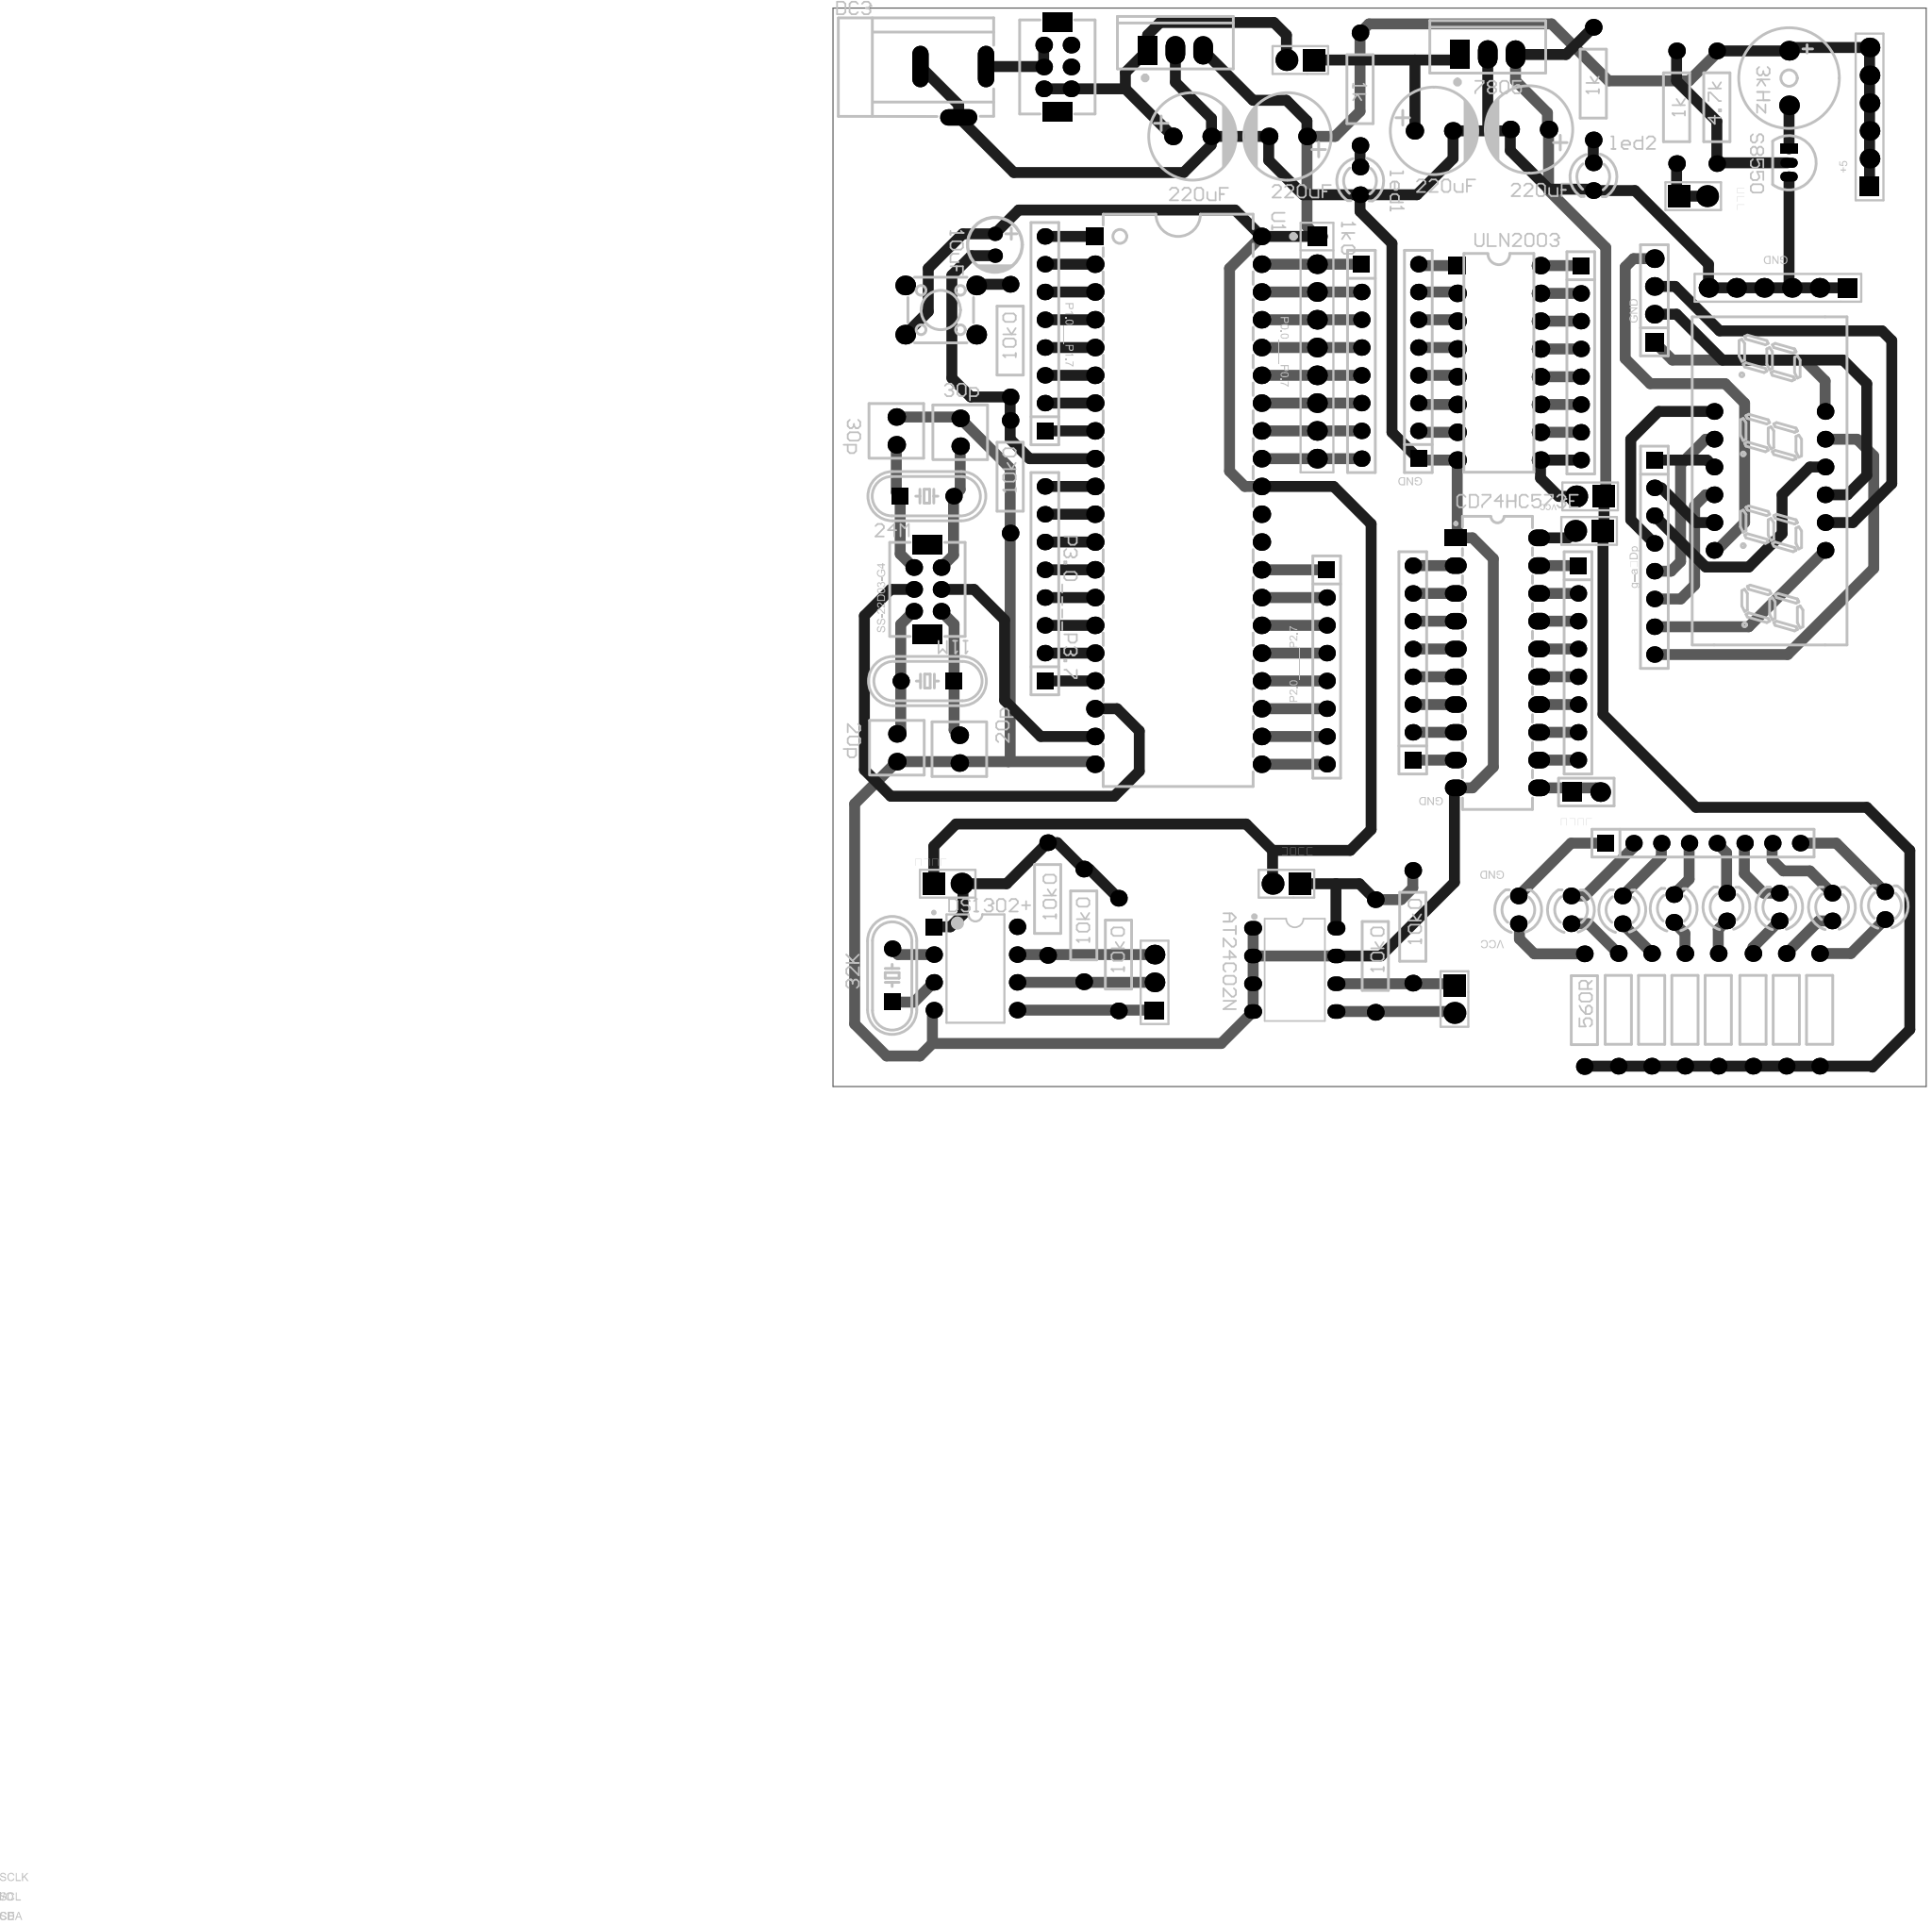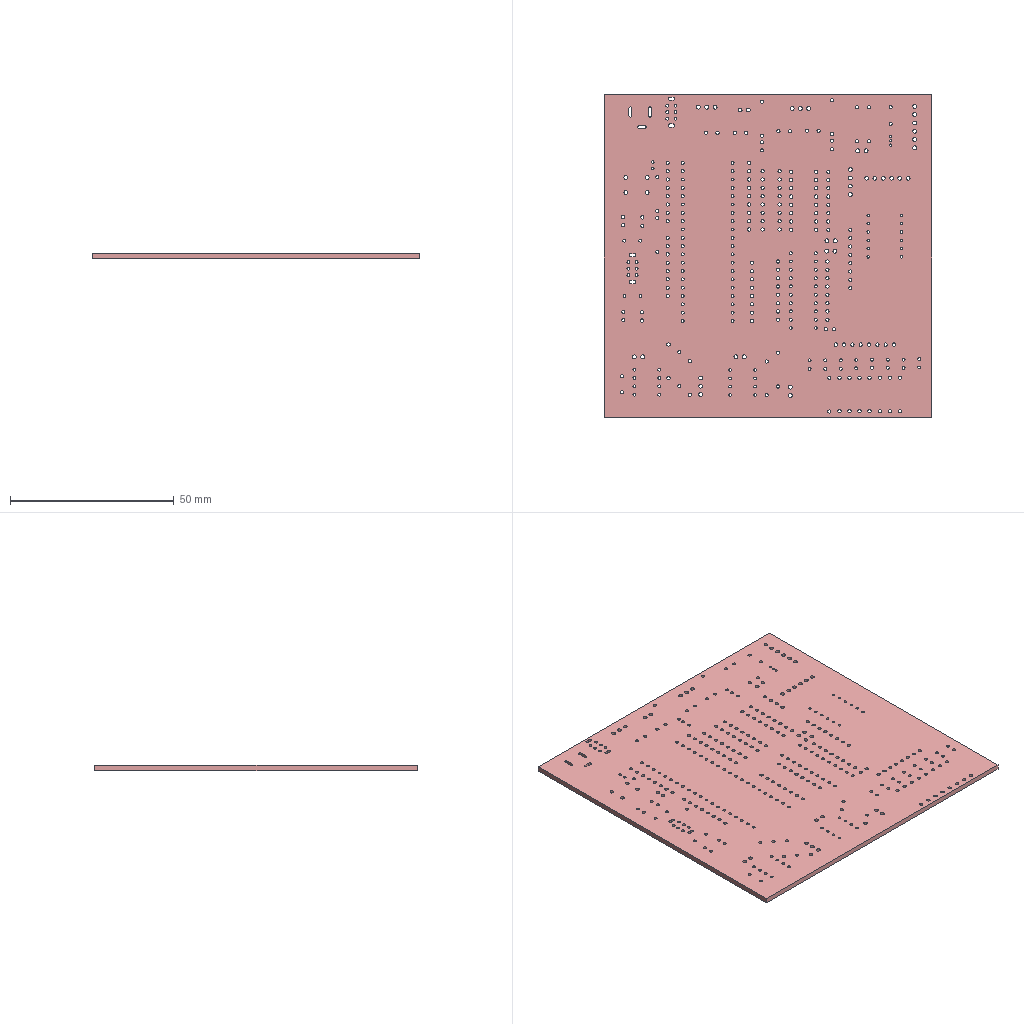Circuit board layout | Altium Designer | box 100 x 98.6 x 1.6 mm
Layer stack:
# Altium Designer layer stack of  (unit mm; dielectric type: 0 none, 1 core, 2 prepreg, 3 surface material)
index,name,kind,layer,copper_thickness_mm,dielectric_type,dielectric_thickness_mm,dielectric_material,dielectric_constant
0,Top Paste Mask Layer,other,,,,,,
1,Top Silkscreen Layer,other,,,,,,
2,Top Solder Mask Layer,dielectric,,,3,0.01,,3.3
3,Top Layer,copper,Top Layer,0.035,,,,
4,Dielectric1,dielectric,,,3,1.51,FR4,4.5
5,Bottom Layer,copper,Bottom Layer,0.035,,,,
6,Bottom Solder Mask Layer,dielectric,,,3,0.01,,3.3
7,Bottom Silkscreen Layer,other,,,,,,
8,Bottom Paste Mask Layer,other,,,,,,
# drill layer pairs: low layer,high layer
drill_pair,Top Layer,Bottom Layer
Part placement:
Designator,Comment,Layer,Footprint,Center-X(mm),Center-Y(mm),Rotation
H31,PZ254V-11-02P,TopLayer,HDR-TH_2P-P2.54-V-M,145.364,127,180
U1,STC89C52RC-40I-PDIP40,TopLayer,DIP-40_L52.0-W13.7-P2.54-LS15.2-BL,107.772,129.794,270
H32,PZ254V-11-02P,TopLayer,HDR-TH_2P-P2.54-V-M,145.458,130.153,180
Q1,ULN2003,TopLayer,DIP-16_L19.8-W6.5-P2.54-LS7.6-BL,137.109,142.367,270
U2,7805,TopLayer,TO-220-3_L10.0-W4.5-P2.54-L,136.093,170.561,0
U3,7805,TopLayer,TO-220-3_L10.0-W4.5-P2.54-L,107.518,170.942,0
U4,DS1302+,TopLayer,DIP-8_L9.8-W6.6-P2.54-LS7.6-BL,89.23,86.995,270
X1,24M,TopLayer,HC-49US_L11.5-W4.5-P4.88,84.785,130.175,0
U5,AT24C02N,TopLayer,DIP-8_L9.2-W6.3-P2.54-LS7.62-BL,118.44,86.868,270
U6,CD74HC573E,TopLayer,DIP-20_L26.8-W6.4-P2.54-LS7.6-BL,136.982,114.935,270
BUZZER1,3kHz,TopLayer,BUZ-TH_BD9.0-P5.00-D0.6-FD,163.652,168.402,270
H16,P3.0____P3.7,TopLayer,HDR-TH_8P-P2.54-V-M,95.58,122.174,90
Q2,S8550,TopLayer,TO-92-3_L4.9-W3.7-P1.27-L,163.652,160.655,270
C1,10uF,TopLayer,CAP-TH_BD5.0-P2.00-D0.8-FD,91.008,153.162,270
SW3,SS-22D03-G4,TopLayer,SW-TH_SS-22D03-G4,96.723,169.418,90
C2,220uF,TopLayer,CAP-TH_BD8.0-P3.50-D0.6-FD,109.042,163.068,0
C3,220uF,TopLayer,CAP-TH_BD8.0-P3.50-D0.6-FD,117.805,163.068,180
LED11,FJ3461AH,TopLayer,LED-SEG-TH_12P-L30.0-W14.0-P2.54-S10.16-BL,161.874,131.572,270
C4,220uF,TopLayer,CAP-TH_BD8.0-P3.50-D0.6-FD,139.903,163.703,180
C5,220uF,TopLayer,CAP-TH_BD8.0-P3.50-D0.6-FD,131.14,163.576,0
LED1,204-10SURD/S530-A3-L,TopLayer,LED-TH_BD3.0-P2.54-FD,153.114,92.483,90
LED2,204-10SURD/S530-A3-L,TopLayer,LED-TH_BD3.0-P2.54-FD,148.415,92.356,90
LED3,led1,TopLayer,LED-TH_BD3.0-P2.54-FD,124.409,159.004,270
LED4,led2,TopLayer,LED-TH_BD3.0-P2.54-FD,145.745,159.385,270
LED5,204-10SURD/S530-A3-L,TopLayer,LED-TH_BD3.0-P2.54-FD,157.94,92.61,90
LED6,204-10SURD/S530-A3-L,TopLayer,LED-TH_BD3.0-P2.54-FD,167.592,92.61,90
LED7,204-10SURD/S530-A3-L,TopLayer,LED-TH_BD3.0-P2.54-FD,172.418,92.737,90
LED8,204-10SURD/S530-A3-L,TopLayer,LED-TH_BD3.0-P2.54-FD,143.716,92.356,90
LED9,204-10SURD/S530-A3-L,TopLayer,LED-TH_BD3.0-P2.54-FD,138.89,92.356,90
LED10,204-10SURD/S530-A3-L,TopLayer,LED-TH_BD3.0-P2.54-FD,162.766,92.61,90
R1,10kΩ,TopLayer,RES-TH_BD2.4-L6.3-P10.30-D0.6,92.405,131.953,90
R2,560R,TopLayer,RES-TH_BD2.4-L6.3-P10.30-D0.6,144.93,83.182,90
R3,10kΩ,TopLayer,RES-TH_BD2.4-L6.3-P10.30-D0.6,99.136,90.932,90
R4,10kΩ,TopLayer,RES-TH_BD2.4-L6.3-P10.30-D0.6,92.405,144.399,90
R5,1k,TopLayer,RES-TH_BD2.4-L6.3-P10.30-D0.6,124.409,167.386,270
R6,10kΩ,TopLayer,RES-TH_BD2.4-L6.3-P10.30-D0.6,95.834,93.345,90
R7,10kΩ,TopLayer,RES-TH_BD2.4-L6.3-P10.30-D0.6,125.806,88.138,90
R8,560R,TopLayer,RES-TH_BD2.4-L6.3-P10.30-D0.6,154.13,83.212,90
R9,10kΩ,TopLayer,RES-TH_BD2.4-L6.3-P10.30-D0.6,102.311,88.265,90
R10,560R,TopLayer,RES-TH_BD2.4-L6.3-P10.30-D0.6,148.034,83.212,90
R11,10kΩ,TopLayer,RES-TH_BD2.4-L6.3-P10.30-D0.6,129.235,90.805,90
R12,560R,TopLayer,RES-TH_BD2.4-L6.3-P10.30-D0.6,157.178,83.212,90
R13,560R,TopLayer,RES-TH_BD2.4-L6.3-P10.30-D0.6,160.353,83.212,90
R14,560R,TopLayer,RES-TH_BD2.4-L6.3-P10.30-D0.6,151.082,83.212,90
H6,GND,TopLayer,HDR-TH_6P-P2.54-V-M-1,162.636,149.225,180
H7,+5,TopLayer,HDR-TH_6P-P2.54-V-M-1,171.018,164.846,90
H11,SCL
SDA,TopLayer,HDR-TH_2P-P2.54-V-M,133.045,84.201,270
H12,蜂鸣器,TopLayer,HDR-TH_2P-P2.54-V-M,154.889,157.607,0
R15,1kΩ,TopLayer,RES-ARRAY-TH_9P-L22.8-W3.00-P2.54,120.472,143.764,270
X2,11M,TopLayer,HC-49US_L11.5-W4.5-P4.88,84.835,113.27,180
DC3,DC-005-20A,TopLayer,DC-IN-TH_DC-005-20A,87.198,167.132,0
X3,32K,TopLayer,HC-49US_L11.5-W4.5-P4.88,81.61,86.36,90
C6,30p,TopLayer,CAP-TH_L5.0-W5.0-P2.54-D1.0,87.833,136.017,270
C7,30p,TopLayer,CAP-TH_L5.0-W5.0-P2.54-D1.0,81.991,136.144,270
C8,20p,TopLayer,CAP-TH_L5.0-W5.0-P2.54-D1.0,82.041,107.174,270
C9,20p,TopLayer,CAP-TH_L5.0-W5.0-P2.54-D1.0,87.756,107.047,90
SW1,TS-1095-A7B2-D1,TopLayer,SW-TH_4P-L6.0-W6.0-P4.50-LS6.5,86.055,147.193,0
SW2,SS-22D03-G4,TopLayer,SW-TH_SS-22D03-G4,84.835,121.652,270
H15,P1.0___P1.7,TopLayer,HDR-TH_8P-P2.54-V-M,95.58,145.034,90
H17,P2.0_____P2.7,TopLayer,HDR-TH_8P-P2.54-V-M,121.361,114.554,270
H18,P0.0____P0.7,TopLayer,HDR-TH_8P-P2.54-V-M,124.536,142.494,270
H19,PZ254V-11-08P,TopLayer,HDR-TH_8P-P2.54-V-M,129.743,142.494,90
R16,1k,TopLayer,RES-TH_BD2.4-L6.3-P10.30-D0.6,145.745,167.894,90
H20,SCLK
I/O
CE,TopLayer,HDR-TH_3P-P2.54-V-M-1,105.613,85.725,90
H21,PZ254V-11-08P,TopLayer,HDR-TH_8P-P2.54-V-M,144.602,142.367,270
H22,数码管口,TopLayer,HDR-TH_2P-P2.54-V-M-1,145.11,103.124,0
H23,PZ254V-11-08P,TopLayer,HDR-TH_8P-P2.54-V-M,129.235,114.935,90
H24,PZ254V-11-08P,TopLayer,HDR-TH_8P-P2.54-V-M,144.348,114.935,270
H25,g--a、Dp,TopLayer,HDR-TH_8P-P2.54-V-M,151.333,124.587,270
H26,GND,TopLayer,HDR-TH_4P-P2.54-V-M,151.333,148.082,90
R17,560R,TopLayer,RES-TH_BD2.4-L6.3-P10.30-D0.6,163.401,83.212,90
R18,560R,TopLayer,RES-TH_BD2.4-L6.3-P10.30-D0.6,166.449,83.212,90
H27,PZ254V-11-08P,TopLayer,HDR-TH_8P-P2.54-V-M,155.781,98.452,0
R19,1k,TopLayer,RES-TH_BD2.4-L6.3-P10.30-D0.6,153.365,165.735,90
R20,4.7k,TopLayer,RES-TH_BD2.4-L6.3-P10.30-D0.6,157.048,165.735,90
H28,PZ254V-11-02P,TopLayer,HDR-TH_2P-P2.54-V-M,118.948,170.053,180
H29,存储电源,TopLayer,HDR-TH_2P-P2.54-V-M,117.678,94.742,180
H30,时钟电源,TopLayer,HDR-TH_2P-P2.54-V-M,86.69,94.742,0
Pad and via stacks:
# Altium Designer via and pad stacks of  (unit mm). Each distinct definition once, with the count of objects using it.
# via: kind,start_layer,end_layer,hole_mm,diameter_mm,mode(0 simple;1 top-mid-bottom;2 full stack),diameter_per_layer,count,example_net
# pad: kind,layer,hole_mm,hole_type(0 round;1 square;2 slot),plating,top_size,top_shape(1 round;2 rect;3 octagon;9 rounded rect),mid_size,bottom_size,mode,footprint,size_per_layer,count,example
pad,Multi-Layer,1.2,0,plated,2x2,2,2x2,2x2,0,HDR-TH_2P-P2.54-V-M,,7,H31.1
pad,Multi-Layer,1.2,0,plated,2x2,1,2x2,2x2,0,HDR-TH_2P-P2.54-V-M,,7,H31.2
pad,Multi-Layer,0.889,0,plated,1.6x1.6,1,1.6x1.6,1.6x1.6,0,DIP-40_L52.0-W13.7-P2.54-LS15.2-BL,,39,U1.31
pad,Multi-Layer,0.889,0,plated,1.6x1.6,2,1.6x1.6,1.6x1.6,0,DIP-40_L52.0-W13.7-P2.54-LS15.2-BL,,1,U1.1
pad,Multi-Layer,1,0,plated,1.6x1.6,1,1.6x1.6,1.6x1.6,0,DIP-16_L19.8-W6.5-P2.54-LS7.6-BL,,15,Q1.16
pad,Multi-Layer,1,0,plated,1.6x1.6,2,1.6x1.6,1.6x1.6,0,DIP-16_L19.8-W6.5-P2.54-LS7.6-BL,,1,Q1.1
pad,Multi-Layer,1.2,0,plated,1.8x2.6,1,1.8x2.6,1.8x2.6,0,TO-220-3_L10.0-W4.5-P2.54-L,,4,U2.2
pad,Multi-Layer,1.2,0,plated,1.8x2.6,2,1.8x2.6,1.8x2.6,0,TO-220-3_L10.0-W4.5-P2.54-L,,2,U2.1
pad,Multi-Layer,0.9,0,plated,1.5x1.5,2,1.5x1.5,1.5x1.5,0,DIP-8_L9.8-W6.6-P2.54-LS7.6-BL,,1,U4.1
pad,Multi-Layer,0.9,0,plated,1.5x1.5,1,1.5x1.5,1.5x1.5,0,DIP-8_L9.8-W6.6-P2.54-LS7.6-BL,,7,U4.2
pad,Multi-Layer,0.9,0,plated,1.5x1.5,2,1.5x1.5,1.5x1.5,0,HC-49US_L11.5-W4.5-P4.88,,3,X1.1
pad,Multi-Layer,0.9,0,plated,1.5x1.5,1,1.5x1.5,1.5x1.5,0,HC-49US_L11.5-W4.5-P4.88,,3,X1.2
pad,Multi-Layer,0.8,0,plated,1.32x1.65,1,1.32x1.65,1.32x1.65,0,DIP-8_L9.2-W6.3-P2.54-LS7.62-BL,,8,U5.1
pad,Multi-Layer,0.9,0,plated,2x1.5,1,2x1.5,2x1.5,0,DIP-20_L26.8-W6.4-P2.54-LS7.6-BL,,8,U6.9
pad,Multi-Layer,0.9,0,plated,2x1.5,2,2x1.5,2x1.5,0,DIP-20_L26.8-W6.4-P2.54-LS7.6-BL,,1,U6.1
pad,Multi-Layer,0.9,0,plated,2x1.524,1,2x1.524,2x1.524,0,DIP-20_L26.8-W6.4-P2.54-LS7.6-BL,,11,U6.10
pad,Multi-Layer,1,0,plated,1.8x1.8,1,1.8x1.8,1.8x1.8,0,BUZ-TH_BD9.0-P5.00-D0.6-FD,,2,BUZZER1.1
pad,Multi-Layer,1,0,plated,1.5x1.5,2,1.5x1.5,1.5x1.5,0,HDR-TH_8P-P2.54-V-M,,10,H16.1
pad,Multi-Layer,1,0,plated,1.5x1.5,1,1.5x1.5,1.5x1.5,0,HDR-TH_8P-P2.54-V-M,,70,H16.2
pad,Multi-Layer,0.7,0,plated,0.9x1.6,1,0.9x1.6,0.9x1.6,0,TO-92-3_L4.9-W3.7-P1.27-L,,2,Q2.3
pad,Multi-Layer,0.7,0,plated,0.9x1.6,2,0.9x1.6,0.9x1.6,0,TO-92-3_L4.9-W3.7-P1.27-L,,1,Q2.1
pad,Multi-Layer,0.8,0,plated,1.3x1.3,1,1.3x1.3,1.3x1.3,0,CAP-TH_BD5.0-P2.00-D0.8-FD,,2,C1.1
pad,Multi-Layer,1.016,2,plated,1.778x2.7,2,1.778x2.7,1.778x2.7,0,SW-TH_SS-22D03-G4,,4,SW3.8
pad,Multi-Layer,0.889,0,plated,1.524x1.524,1,1.524x1.524,1.524x1.524,0,SW-TH_SS-22D03-G4,,12,SW3.4
pad,Multi-Layer,1,0,plated,1.6x1.6,1,1.6x1.6,1.6x1.6,0,CAP-TH_BD8.0-P3.50-D0.6-FD,,8,C2.2
pad,Multi-Layer,0.762,0,plated,1.524x1.524,1,1.524x1.524,1.524x1.524,0,LED-SEG-TH_12P-L30.0-W14.0-P2.54-S10.16-BL,,12,LED11.12
pad,Multi-Layer,0.9144,0,plated,1.524x1.524,1,1.524x1.524,1.524x1.524,0,LED-TH_BD3.0-P2.54-FD,,20,LED1.1
pad,Multi-Layer,1,0,plated,1.524x1.524,1,1.524x1.524,1.524x1.524,0,RES-TH_BD2.4-L6.3-P10.30-D0.6,,38,R1.1
pad,Multi-Layer,1.2,0,plated,1.8x1.8,1,1.8x1.8,1.8x1.8,0,HDR-TH_6P-P2.54-V-M-1,,10,H6.6
pad,Multi-Layer,1.2,0,plated,1.8x1.8,2,1.8x1.8,1.8x1.8,0,HDR-TH_6P-P2.54-V-M-1,,2,H6.1
pad,Multi-Layer,1,0,plated,1.8x1.8,2,1.8x1.8,1.8x1.8,0,RES-ARRAY-TH_9P-L22.8-W3.00-P2.54,,1,R15.1
pad,Multi-Layer,1,0,plated,1.8x1.8,1,1.8x1.8,1.8x1.8,0,RES-ARRAY-TH_9P-L22.8-W3.00-P2.54,,8,R15.2
pad,Multi-Layer,0.9,2,plated,1.5x3.8,1,1.5x3.8,1.5x3.8,0,DC-IN-TH_DC-005-20A,,2,DC3.1
pad,Multi-Layer,0.9,2,plated,1.5x3.4,1,1.5x3.4,1.5x3.4,0,DC-IN-TH_DC-005-20A,,1,DC3.3
pad,Multi-Layer,1,0,plated,1.6x1.6,1,1.6x1.6,1.6x1.6,0,CAP-TH_L5.0-W5.0-P2.54-D1.0,,8,C6.1
pad,Multi-Layer,1.2,0,plated,1.8x1.8,1,1.8x1.8,1.8x1.8,0,SW-TH_4P-L6.0-W6.0-P4.50-LS6.5,,4,SW1.1
pad,Multi-Layer,1.2,0,plated,1.8x1.8,1,1.8x1.8,1.8x1.8,0,HDR-TH_3P-P2.54-V-M-1,,2,H20.3
pad,Multi-Layer,1.2,0,plated,1.575x1.8,2,1.575x1.8,1.575x1.8,0,HDR-TH_3P-P2.54-V-M-1,,1,H20.1
pad,Multi-Layer,1,0,plated,1.8x1.8,1,1.8x1.8,1.8x1.8,0,HDR-TH_2P-P2.54-V-M-1,,1,H22.2
pad,Multi-Layer,1,0,plated,1.8x1.8,2,1.8x1.8,1.8x1.8,0,HDR-TH_2P-P2.54-V-M-1,,1,H22.1
pad,Multi-Layer,1.1,0,plated,1.7x1.7,2,1.7x1.7,1.7x1.7,0,HDR-TH_4P-P2.54-V-M,,1,H26.1
pad,Multi-Layer,1.1,0,plated,1.7x1.7,1,1.7x1.7,1.7x1.7,0,HDR-TH_4P-P2.54-V-M,,3,H26.2
Design rules, without the lines most boards share:
# Altium Designer design rules of  (exported by Altium Designer, unit mm)
# columns: name | kind | enabled | priority | scope1 | scope2 | descriptor | typed fields (field=value)
otherClearance | 52 | enabled | 1 | All | All | Hole To Hole Clearance (Gap=11.8mil) (All),(All) | gap=0.2997